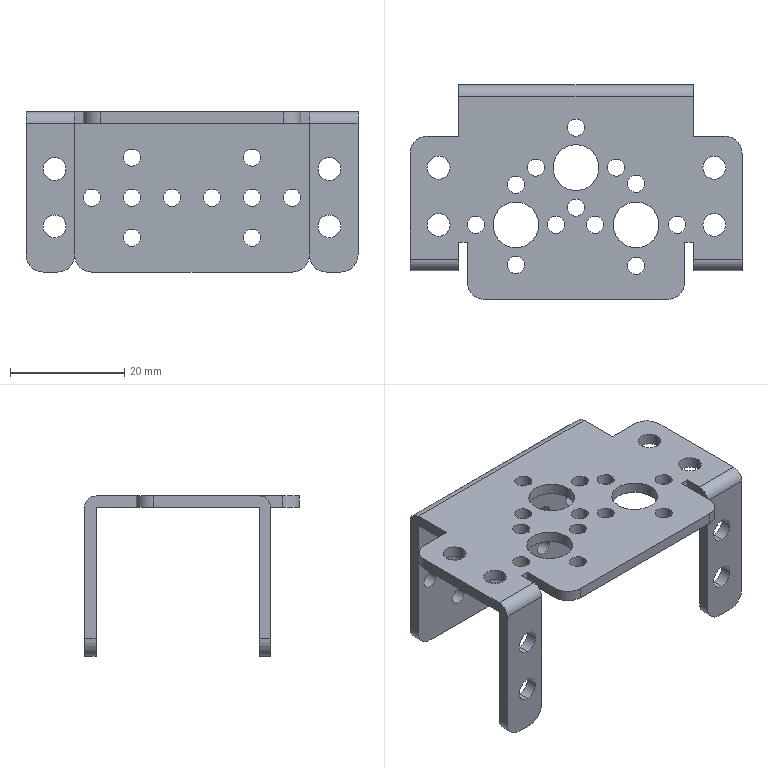Part | STEP file | Multifunction bracket | 2 solids | 106 faces | box 58 x 37.5 x 28 mm | volume 5928 mm3 | cylinder 79 | plane 27 | commonest cylinder face diameters 3 x44 4 x19 6 x10 8 x6